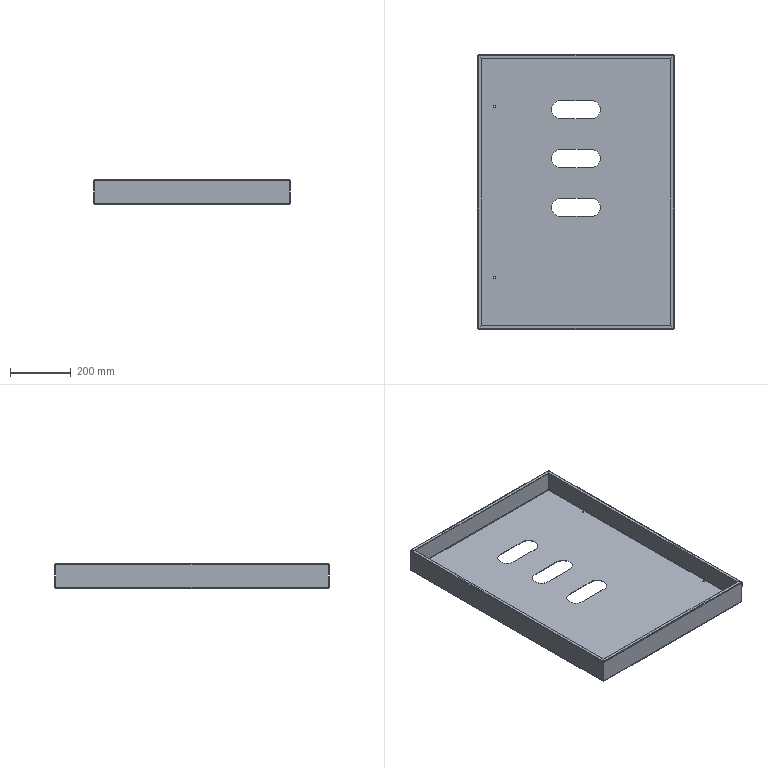Part | SolidWorks | features EdgeFlange 2, ICE 2, FlatPattern 1, SMBaseFlange 1, SheetMetal 1 | 1 solid | 93 faces | box 645 x 900 x 80 mm | volume 1637213 mm3 | plane 44 | cylinder 33 | spline 16 | commonest cylinder face diameters 6 x16 60 x9 2 x8